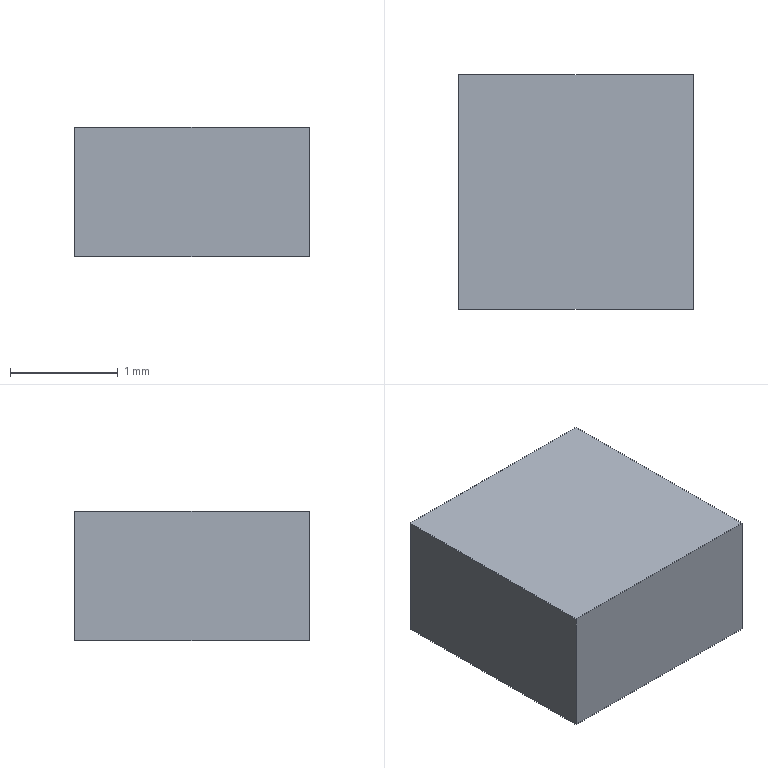Part | Creo | 1 solid | 6 faces | box 2.175 x 2.175 x 1.2 mm | volume 5.677 mm3 | plane 6
STEP:
#1=CARTESIAN_POINT('',(0.,0.,0.));
#2=DIRECTION('',(0.,0.,1.));
#3=DIRECTION('',(1.,0.,0.));
#4=AXIS2_PLACEMENT_3D('',#1,#2,#3);
#5=CARTESIAN_POINT('',(-1.15,-1.025,0.));
#6=VERTEX_POINT('',#5);
#7=CARTESIAN_POINT('',(1.025,-1.025,0.));
#8=VERTEX_POINT('',#7);
#9=CARTESIAN_POINT('',(-1.15,-1.025,0.));
#10=DIRECTION('',(1.,0.,0.));
#11=VECTOR('',#10,2.175);
#12=LINE('',#9,#11);
#13=EDGE_CURVE('',#6,#8,#12,.T.);
#14=ORIENTED_EDGE('',*,*,#13,.T.);
#15=CARTESIAN_POINT('',(1.025,1.15,0.));
#16=VERTEX_POINT('',#15);
#17=CARTESIAN_POINT('',(1.025,-1.025,0.));
#18=DIRECTION('',(0.,1.,0.));
#19=VECTOR('',#18,2.175);
#20=LINE('',#17,#19);
#21=EDGE_CURVE('',#8,#16,#20,.T.);
#22=ORIENTED_EDGE('',*,*,#21,.T.);
#23=CARTESIAN_POINT('',(-1.15,1.15,0.));
#24=VERTEX_POINT('',#23);
#25=CARTESIAN_POINT('',(1.025,1.15,0.));
#26=DIRECTION('',(-1.,0.,0.));
#27=VECTOR('',#26,2.175);
#28=LINE('',#25,#27);
#29=EDGE_CURVE('',#16,#24,#28,.T.);
#30=ORIENTED_EDGE('',*,*,#29,.T.);
#31=CARTESIAN_POINT('',(-1.15,1.15,0.));
#32=DIRECTION('',(0.,-1.,0.));
#33=VECTOR('',#32,2.175);
#34=LINE('',#31,#33);
#35=EDGE_CURVE('',#24,#6,#34,.T.);
#36=ORIENTED_EDGE('',*,*,#35,.T.);
#37=EDGE_LOOP('',(#14,#22,#30,#36));
#38=FACE_OUTER_BOUND('',#37,.F.);
#39=CARTESIAN_POINT('',(0.,0.,0.));
#40=DIRECTION('',(0.,0.,1.));
#41=DIRECTION('',(1.,0.,0.));
#42=AXIS2_PLACEMENT_3D('',#39,#40,#41);
#43=PLANE('',#42);
#44=ADVANCED_FACE('',(#38),#43,.F.);
#45=ORIENTED_EDGE('',*,*,#13,.F.);
#46=CARTESIAN_POINT('',(-1.15,-1.025,1.2));
#47=VERTEX_POINT('',#46);
#48=CARTESIAN_POINT('',(-1.15,-1.025,0.));
#49=DIRECTION('',(0.,0.,1.));
#50=VECTOR('',#49,1.2);
#51=LINE('',#48,#50);
#52=EDGE_CURVE('',#6,#47,#51,.T.);
#53=ORIENTED_EDGE('',*,*,#52,.T.);
#54=CARTESIAN_POINT('',(1.025,-1.025,1.2));
#55=VERTEX_POINT('',#54);
#56=CARTESIAN_POINT('',(-1.15,-1.025,1.2));
#57=DIRECTION('',(1.,0.,0.));
#58=VECTOR('',#57,2.175);
#59=LINE('',#56,#58);
#60=EDGE_CURVE('',#47,#55,#59,.T.);
#61=ORIENTED_EDGE('',*,*,#60,.T.);
#62=CARTESIAN_POINT('',(1.025,-1.025,0.));
#63=DIRECTION('',(0.,0.,1.));
#64=VECTOR('',#63,1.2);
#65=LINE('',#62,#64);
#66=EDGE_CURVE('',#8,#55,#65,.T.);
#67=ORIENTED_EDGE('',*,*,#66,.F.);
#68=EDGE_LOOP('',(#45,#53,#61,#67));
#69=FACE_OUTER_BOUND('',#68,.F.);
#70=CARTESIAN_POINT('',(-1.15,-1.025,0.));
#71=DIRECTION('',(0.,-1.,0.));
#72=DIRECTION('',(1.,0.,0.));
#73=AXIS2_PLACEMENT_3D('',#70,#71,#72);
#74=PLANE('',#73);
#75=ADVANCED_FACE('',(#69),#74,.T.);
#76=ORIENTED_EDGE('',*,*,#35,.F.);
#77=CARTESIAN_POINT('',(-1.15,1.15,1.2));
#78=VERTEX_POINT('',#77);
#79=CARTESIAN_POINT('',(-1.15,1.15,0.));
#80=DIRECTION('',(0.,0.,1.));
#81=VECTOR('',#80,1.2);
#82=LINE('',#79,#81);
#83=EDGE_CURVE('',#24,#78,#82,.T.);
#84=ORIENTED_EDGE('',*,*,#83,.T.);
#85=CARTESIAN_POINT('',(-1.15,1.15,1.2));
#86=DIRECTION('',(0.,-1.,0.));
#87=VECTOR('',#86,2.175);
#88=LINE('',#85,#87);
#89=EDGE_CURVE('',#78,#47,#88,.T.);
#90=ORIENTED_EDGE('',*,*,#89,.T.);
#91=ORIENTED_EDGE('',*,*,#52,.F.);
#92=EDGE_LOOP('',(#76,#84,#90,#91));
#93=FACE_OUTER_BOUND('',#92,.F.);
#94=CARTESIAN_POINT('',(-1.15,1.15,0.));
#95=DIRECTION('',(-1.,0.,0.));
#96=DIRECTION('',(0.,-1.,0.));
#97=AXIS2_PLACEMENT_3D('',#94,#95,#96);
#98=PLANE('',#97);
#99=ADVANCED_FACE('',(#93),#98,.T.);
#100=ORIENTED_EDGE('',*,*,#29,.F.);
#101=CARTESIAN_POINT('',(1.025,1.15,1.2));
#102=VERTEX_POINT('',#101);
#103=CARTESIAN_POINT('',(1.025,1.15,0.));
#104=DIRECTION('',(0.,0.,1.));
#105=VECTOR('',#104,1.2);
#106=LINE('',#103,#105);
#107=EDGE_CURVE('',#16,#102,#106,.T.);
#108=ORIENTED_EDGE('',*,*,#107,.T.);
#109=CARTESIAN_POINT('',(1.025,1.15,1.2));
#110=DIRECTION('',(-1.,0.,0.));
#111=VECTOR('',#110,2.175);
#112=LINE('',#109,#111);
#113=EDGE_CURVE('',#102,#78,#112,.T.);
#114=ORIENTED_EDGE('',*,*,#113,.T.);
#115=ORIENTED_EDGE('',*,*,#83,.F.);
#116=EDGE_LOOP('',(#100,#108,#114,#115));
#117=FACE_OUTER_BOUND('',#116,.F.);
#118=CARTESIAN_POINT('',(1.025,1.15,0.));
#119=DIRECTION('',(0.,1.,0.));
#120=DIRECTION('',(-1.,0.,0.));
#121=AXIS2_PLACEMENT_3D('',#118,#119,#120);
#122=PLANE('',#121);
#123=ADVANCED_FACE('',(#117),#122,.T.);
#124=ORIENTED_EDGE('',*,*,#21,.F.);
#125=ORIENTED_EDGE('',*,*,#66,.T.);
#126=CARTESIAN_POINT('',(1.025,-1.025,1.2));
#127=DIRECTION('',(0.,1.,0.));
#128=VECTOR('',#127,2.175);
#129=LINE('',#126,#128);
#130=EDGE_CURVE('',#55,#102,#129,.T.);
#131=ORIENTED_EDGE('',*,*,#130,.T.);
#132=ORIENTED_EDGE('',*,*,#107,.F.);
#133=EDGE_LOOP('',(#124,#125,#131,#132));
#134=FACE_OUTER_BOUND('',#133,.F.);
#135=CARTESIAN_POINT('',(1.025,-1.025,0.));
#136=DIRECTION('',(1.,0.,0.));
#137=DIRECTION('',(0.,1.,0.));
#138=AXIS2_PLACEMENT_3D('',#135,#136,#137);
#139=PLANE('',#138);
#140=ADVANCED_FACE('',(#134),#139,.T.);
#141=ORIENTED_EDGE('',*,*,#60,.F.);
#142=ORIENTED_EDGE('',*,*,#89,.F.);
#143=ORIENTED_EDGE('',*,*,#113,.F.);
#144=ORIENTED_EDGE('',*,*,#130,.F.);
#145=EDGE_LOOP('',(#141,#142,#143,#144));
#146=FACE_OUTER_BOUND('',#145,.F.);
#147=CARTESIAN_POINT('',(0.,0.,1.2));
#148=DIRECTION('',(0.,0.,1.));
#149=DIRECTION('',(1.,0.,0.));
#150=AXIS2_PLACEMENT_3D('',#147,#148,#149);
#151=PLANE('',#150);
#152=ADVANCED_FACE('',(#146),#151,.T.);
#153=CLOSED_SHELL('',(#44,#75,#99,#123,#140,#152));
#154=MANIFOLD_SOLID_BREP('',#153);
#155=(LENGTH_UNIT()NAMED_UNIT(*)SI_UNIT(.MILLI.,.METRE.));
#156=UNCERTAINTY_MEASURE_WITH_UNIT(LENGTH_MEASURE(0.0003302),#155,'','');
#157=(NAMED_UNIT(*)PLANE_ANGLE_UNIT()SI_UNIT($,.RADIAN.));
#158=PLANE_ANGLE_MEASURE_WITH_UNIT(PLANE_ANGLE_MEASURE(0.01745),#157);
#159=(CONVERSION_BASED_UNIT('DEGREE',#158)NAMED_UNIT(*)PLANE_ANGLE_UNIT());
#160=(NAMED_UNIT(*)SI_UNIT($,.STERADIAN.)SOLID_ANGLE_UNIT());
#161=(GEOMETRIC_REPRESENTATION_CONTEXT(3)GLOBAL_UNCERTAINTY_ASSIGNED_CONTEXT((#156))GLOBAL_UNIT_ASSIGNED_CONTEXT((#155,#159,#160))REPRESENTATION_CONTEXT('',''));
#162=ADVANCED_BREP_SHAPE_REPRESENTATION('',(#4,#154),#161);